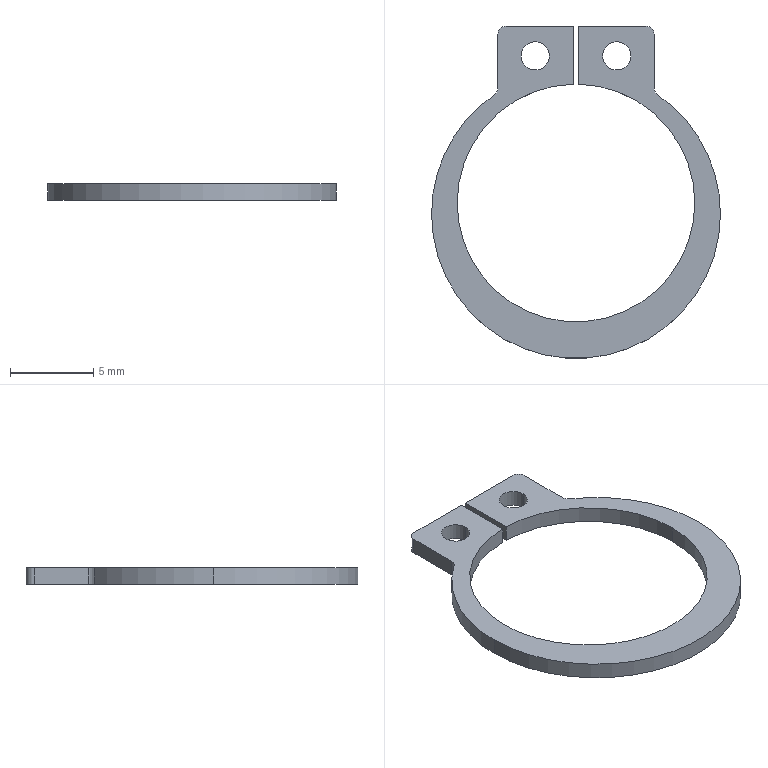Part | SolidWorks | features BaseBody 1 | 1 solid | 22 faces | box 17.38 x 20 x 1 mm | volume 99.766 mm3 | cylinder 14 | plane 8 | commonest cylinder face diameters 1 x4 1.7 x4 14.3 x3 17.38 x3
STEP:
#1=CARTESIAN_POINT('',(-130.796,1840.394,-232.));
#2=VERTEX_POINT('',#1);
#3=CARTESIAN_POINT('',(-129.096,1840.394,-232.));
#4=VERTEX_POINT('',#3);
#5=CARTESIAN_POINT('',(-129.946,1840.394,-232.));
#6=DIRECTION('',(0.,0.,1.));
#7=DIRECTION('',(1.,0.,0.));
#8=AXIS2_PLACEMENT_3D('',#5,#6,#7);
#9=CIRCLE('',#8,0.85);
#10=EDGE_CURVE('',#2,#4,#9,.T.);
#11=ORIENTED_EDGE('',*,*,#10,.F.);
#12=CARTESIAN_POINT('',(-130.796,1840.394,-231.));
#13=VERTEX_POINT('',#12);
#14=CARTESIAN_POINT('',(-130.796,1840.394,-232.));
#15=DIRECTION('',(0.,0.,1.));
#16=VECTOR('',#15,1000.);
#17=LINE('',#14,#16);
#18=EDGE_CURVE('',#2,#13,#17,.T.);
#19=ORIENTED_EDGE('',*,*,#18,.T.);
#20=CARTESIAN_POINT('',(-129.096,1840.394,-231.));
#21=VERTEX_POINT('',#20);
#22=CARTESIAN_POINT('',(-129.946,1840.394,-231.));
#23=DIRECTION('',(0.,0.,1.));
#24=DIRECTION('',(1.,0.,0.));
#25=AXIS2_PLACEMENT_3D('',#22,#23,#24);
#26=CIRCLE('',#25,0.85);
#27=EDGE_CURVE('',#13,#21,#26,.T.);
#28=ORIENTED_EDGE('',*,*,#27,.T.);
#29=CARTESIAN_POINT('',(-129.096,1840.394,-232.));
#30=DIRECTION('',(0.,0.,1.));
#31=VECTOR('',#30,1000.);
#32=LINE('',#29,#31);
#33=EDGE_CURVE('',#4,#21,#32,.T.);
#34=ORIENTED_EDGE('',*,*,#33,.F.);
#35=EDGE_LOOP('',(#11,#19,#28,#34));
#36=FACE_OUTER_BOUND('',#35,.T.);
#37=CARTESIAN_POINT('',(-129.946,1840.394,-232.));
#38=DIRECTION('',(0.,0.,1.));
#39=DIRECTION('',(1.,0.,0.));
#40=AXIS2_PLACEMENT_3D('',#37,#38,#39);
#41=CYLINDRICAL_SURFACE('',#40,0.85);
#42=ADVANCED_FACE('',(#36),#41,.F.);
#43=CARTESIAN_POINT('',(-125.896,1840.394,-232.));
#44=VERTEX_POINT('',#43);
#45=CARTESIAN_POINT('',(-124.196,1840.394,-232.));
#46=VERTEX_POINT('',#45);
#47=CARTESIAN_POINT('',(-125.046,1840.394,-232.));
#48=DIRECTION('',(0.,0.,1.));
#49=DIRECTION('',(1.,0.,0.));
#50=AXIS2_PLACEMENT_3D('',#47,#48,#49);
#51=CIRCLE('',#50,0.85);
#52=EDGE_CURVE('',#44,#46,#51,.T.);
#53=ORIENTED_EDGE('',*,*,#52,.F.);
#54=CARTESIAN_POINT('',(-125.896,1840.394,-231.));
#55=VERTEX_POINT('',#54);
#56=CARTESIAN_POINT('',(-125.896,1840.394,-232.));
#57=DIRECTION('',(0.,0.,1.));
#58=VECTOR('',#57,1000.);
#59=LINE('',#56,#58);
#60=EDGE_CURVE('',#44,#55,#59,.T.);
#61=ORIENTED_EDGE('',*,*,#60,.T.);
#62=CARTESIAN_POINT('',(-124.196,1840.394,-231.));
#63=VERTEX_POINT('',#62);
#64=CARTESIAN_POINT('',(-125.046,1840.394,-231.));
#65=DIRECTION('',(0.,0.,1.));
#66=DIRECTION('',(1.,0.,0.));
#67=AXIS2_PLACEMENT_3D('',#64,#65,#66);
#68=CIRCLE('',#67,0.85);
#69=EDGE_CURVE('',#55,#63,#68,.T.);
#70=ORIENTED_EDGE('',*,*,#69,.T.);
#71=CARTESIAN_POINT('',(-124.196,1840.394,-232.));
#72=DIRECTION('',(0.,0.,1.));
#73=VECTOR('',#72,1000.);
#74=LINE('',#71,#73);
#75=EDGE_CURVE('',#46,#63,#74,.T.);
#76=ORIENTED_EDGE('',*,*,#75,.F.);
#77=EDGE_LOOP('',(#53,#61,#70,#76));
#78=FACE_OUTER_BOUND('',#77,.T.);
#79=CARTESIAN_POINT('',(-125.046,1840.394,-232.));
#80=DIRECTION('',(0.,0.,1.));
#81=DIRECTION('',(1.,0.,0.));
#82=AXIS2_PLACEMENT_3D('',#79,#80,#81);
#83=CYLINDRICAL_SURFACE('',#82,0.85);
#84=ADVANCED_FACE('',(#78),#83,.F.);
#85=CARTESIAN_POINT('',(-132.413,1838.049,-232.));
#86=VERTEX_POINT('',#85);
#87=CARTESIAN_POINT('',(-136.186,1830.884,-232.));
#88=VERTEX_POINT('',#87);
#89=CARTESIAN_POINT('',(-127.496,1830.884,-232.));
#90=DIRECTION('',(0.,0.,1.));
#91=DIRECTION('',(1.,0.,0.));
#92=AXIS2_PLACEMENT_3D('',#89,#90,#91);
#93=CIRCLE('',#92,8.69);
#94=EDGE_CURVE('',#86,#88,#93,.T.);
#95=ORIENTED_EDGE('',*,*,#94,.T.);
#96=CARTESIAN_POINT('',(-136.186,1830.884,-231.));
#97=VERTEX_POINT('',#96);
#98=CARTESIAN_POINT('',(-136.186,1830.884,-232.));
#99=DIRECTION('',(0.,0.,1.));
#100=VECTOR('',#99,1000.);
#101=LINE('',#98,#100);
#102=EDGE_CURVE('',#88,#97,#101,.T.);
#103=ORIENTED_EDGE('',*,*,#102,.T.);
#104=CARTESIAN_POINT('',(-132.413,1838.049,-231.));
#105=VERTEX_POINT('',#104);
#106=CARTESIAN_POINT('',(-127.496,1830.884,-231.));
#107=DIRECTION('',(0.,0.,-1.));
#108=DIRECTION('',(1.,0.,0.));
#109=AXIS2_PLACEMENT_3D('',#106,#107,#108);
#110=CIRCLE('',#109,8.69);
#111=EDGE_CURVE('',#97,#105,#110,.T.);
#112=ORIENTED_EDGE('',*,*,#111,.T.);
#113=CARTESIAN_POINT('',(-132.413,1838.049,-232.));
#114=DIRECTION('',(0.,0.,-1.));
#115=VECTOR('',#114,1000.);
#116=LINE('',#113,#115);
#117=EDGE_CURVE('',#105,#86,#116,.T.);
#118=ORIENTED_EDGE('',*,*,#117,.T.);
#119=EDGE_LOOP('',(#95,#103,#112,#118));
#120=FACE_OUTER_BOUND('',#119,.T.);
#121=CARTESIAN_POINT('',(-127.496,1830.884,-232.));
#122=DIRECTION('',(0.,0.,1.));
#123=DIRECTION('',(1.,0.,0.));
#124=AXIS2_PLACEMENT_3D('',#121,#122,#123);
#125=CYLINDRICAL_SURFACE('',#124,8.69);
#126=ADVANCED_FACE('',(#120),#125,.T.);
#127=ORIENTED_EDGE('',*,*,#102,.F.);
#128=CARTESIAN_POINT('',(-118.806,1830.884,-232.));
#129=VERTEX_POINT('',#128);
#130=CARTESIAN_POINT('',(-127.496,1830.884,-232.));
#131=DIRECTION('',(0.,0.,1.));
#132=DIRECTION('',(1.,0.,0.));
#133=AXIS2_PLACEMENT_3D('',#130,#131,#132);
#134=CIRCLE('',#133,8.69);
#135=EDGE_CURVE('',#88,#129,#134,.T.);
#136=ORIENTED_EDGE('',*,*,#135,.T.);
#137=CARTESIAN_POINT('',(-118.806,1830.884,-231.));
#138=VERTEX_POINT('',#137);
#139=CARTESIAN_POINT('',(-118.806,1830.884,-232.));
#140=DIRECTION('',(0.,0.,1.));
#141=VECTOR('',#140,1000.);
#142=LINE('',#139,#141);
#143=EDGE_CURVE('',#129,#138,#142,.T.);
#144=ORIENTED_EDGE('',*,*,#143,.T.);
#145=CARTESIAN_POINT('',(-127.496,1830.884,-231.));
#146=DIRECTION('',(0.,0.,-1.));
#147=DIRECTION('',(1.,0.,0.));
#148=AXIS2_PLACEMENT_3D('',#145,#146,#147);
#149=CIRCLE('',#148,8.69);
#150=EDGE_CURVE('',#138,#97,#149,.T.);
#151=ORIENTED_EDGE('',*,*,#150,.T.);
#152=EDGE_LOOP('',(#127,#136,#144,#151));
#153=FACE_OUTER_BOUND('',#152,.T.);
#154=CARTESIAN_POINT('',(-127.496,1830.884,-232.));
#155=DIRECTION('',(0.,0.,1.));
#156=DIRECTION('',(1.,0.,0.));
#157=AXIS2_PLACEMENT_3D('',#154,#155,#156);
#158=CYLINDRICAL_SURFACE('',#157,8.69);
#159=ADVANCED_FACE('',(#153),#158,.T.);
#160=CARTESIAN_POINT('',(-134.646,1831.544,-232.));
#161=VERTEX_POINT('',#160);
#162=CARTESIAN_POINT('',(-120.346,1831.544,-232.));
#163=VERTEX_POINT('',#162);
#164=CARTESIAN_POINT('',(-127.496,1831.544,-232.));
#165=DIRECTION('',(0.,0.,1.));
#166=DIRECTION('',(1.,0.,0.));
#167=AXIS2_PLACEMENT_3D('',#164,#165,#166);
#168=CIRCLE('',#167,7.15);
#169=EDGE_CURVE('',#161,#163,#168,.T.);
#170=ORIENTED_EDGE('',*,*,#169,.F.);
#171=CARTESIAN_POINT('',(-134.646,1831.544,-231.));
#172=VERTEX_POINT('',#171);
#173=CARTESIAN_POINT('',(-134.646,1831.544,-232.));
#174=DIRECTION('',(0.,0.,1.));
#175=VECTOR('',#174,1000.);
#176=LINE('',#173,#175);
#177=EDGE_CURVE('',#161,#172,#176,.T.);
#178=ORIENTED_EDGE('',*,*,#177,.T.);
#179=CARTESIAN_POINT('',(-120.346,1831.544,-231.));
#180=VERTEX_POINT('',#179);
#181=CARTESIAN_POINT('',(-127.496,1831.544,-231.));
#182=DIRECTION('',(0.,0.,1.));
#183=DIRECTION('',(1.,0.,0.));
#184=AXIS2_PLACEMENT_3D('',#181,#182,#183);
#185=CIRCLE('',#184,7.15);
#186=EDGE_CURVE('',#172,#180,#185,.T.);
#187=ORIENTED_EDGE('',*,*,#186,.T.);
#188=CARTESIAN_POINT('',(-120.346,1831.544,-232.));
#189=DIRECTION('',(0.,0.,1.));
#190=VECTOR('',#189,1000.);
#191=LINE('',#188,#190);
#192=EDGE_CURVE('',#163,#180,#191,.T.);
#193=ORIENTED_EDGE('',*,*,#192,.F.);
#194=EDGE_LOOP('',(#170,#178,#187,#193));
#195=FACE_OUTER_BOUND('',#194,.T.);
#196=CARTESIAN_POINT('',(-127.496,1831.544,-232.));
#197=DIRECTION('',(0.,0.,1.));
#198=DIRECTION('',(1.,0.,0.));
#199=AXIS2_PLACEMENT_3D('',#196,#197,#198);
#200=CYLINDRICAL_SURFACE('',#199,7.15);
#201=ADVANCED_FACE('',(#195),#200,.F.);
#202=CARTESIAN_POINT('',(-127.346,1838.692,-232.));
#203=VERTEX_POINT('',#202);
#204=CARTESIAN_POINT('',(-127.496,1831.544,-232.));
#205=DIRECTION('',(0.,0.,1.));
#206=DIRECTION('',(1.,0.,0.));
#207=AXIS2_PLACEMENT_3D('',#204,#205,#206);
#208=CIRCLE('',#207,7.15);
#209=EDGE_CURVE('',#163,#203,#208,.T.);
#210=ORIENTED_EDGE('',*,*,#209,.F.);
#211=ORIENTED_EDGE('',*,*,#192,.T.);
#212=CARTESIAN_POINT('',(-127.346,1838.692,-231.));
#213=VERTEX_POINT('',#212);
#214=CARTESIAN_POINT('',(-127.496,1831.544,-231.));
#215=DIRECTION('',(0.,0.,1.));
#216=DIRECTION('',(1.,0.,0.));
#217=AXIS2_PLACEMENT_3D('',#214,#215,#216);
#218=CIRCLE('',#217,7.15);
#219=EDGE_CURVE('',#180,#213,#218,.T.);
#220=ORIENTED_EDGE('',*,*,#219,.T.);
#221=CARTESIAN_POINT('',(-127.346,1838.692,-232.));
#222=DIRECTION('',(0.,0.,1.));
#223=VECTOR('',#222,1000.);
#224=LINE('',#221,#223);
#225=EDGE_CURVE('',#203,#213,#224,.T.);
#226=ORIENTED_EDGE('',*,*,#225,.F.);
#227=EDGE_LOOP('',(#210,#211,#220,#226));
#228=FACE_OUTER_BOUND('',#227,.T.);
#229=CARTESIAN_POINT('',(-127.496,1831.544,-232.));
#230=DIRECTION('',(0.,0.,1.));
#231=DIRECTION('',(1.,0.,0.));
#232=AXIS2_PLACEMENT_3D('',#229,#230,#231);
#233=CYLINDRICAL_SURFACE('',#232,7.15);
#234=ADVANCED_FACE('',(#228),#233,.F.);
#235=CARTESIAN_POINT('',(-129.946,1840.394,-231.));
#236=DIRECTION('',(0.,0.,1.));
#237=DIRECTION('',(1.,0.,0.));
#238=AXIS2_PLACEMENT_3D('',#235,#236,#237);
#239=CIRCLE('',#238,0.85);
#240=EDGE_CURVE('',#21,#13,#239,.T.);
#241=ORIENTED_EDGE('',*,*,#240,.F.);
#242=ORIENTED_EDGE('',*,*,#27,.F.);
#243=EDGE_LOOP('',(#241,#242));
#244=FACE_BOUND('',#243,.T.);
#245=CARTESIAN_POINT('',(-125.046,1840.394,-231.));
#246=DIRECTION('',(0.,0.,1.));
#247=DIRECTION('',(1.,0.,0.));
#248=AXIS2_PLACEMENT_3D('',#245,#246,#247);
#249=CIRCLE('',#248,0.85);
#250=EDGE_CURVE('',#63,#55,#249,.T.);
#251=ORIENTED_EDGE('',*,*,#250,.F.);
#252=ORIENTED_EDGE('',*,*,#69,.F.);
#253=EDGE_LOOP('',(#251,#252));
#254=FACE_BOUND('',#253,.T.);
#255=CARTESIAN_POINT('',(-122.796,1838.461,-231.));
#256=VERTEX_POINT('',#255);
#257=CARTESIAN_POINT('',(-122.579,1838.049,-231.));
#258=VERTEX_POINT('',#257);
#259=CARTESIAN_POINT('',(-122.296,1838.461,-231.));
#260=DIRECTION('',(0.,0.,1.));
#261=DIRECTION('',(1.,0.,0.));
#262=AXIS2_PLACEMENT_3D('',#259,#260,#261);
#263=CIRCLE('',#262,0.5);
#264=EDGE_CURVE('',#256,#258,#263,.T.);
#265=ORIENTED_EDGE('',*,*,#264,.F.);
#266=CARTESIAN_POINT('',(-122.796,1841.694,-231.));
#267=VERTEX_POINT('',#266);
#268=CARTESIAN_POINT('',(-122.796,1838.461,-231.));
#269=DIRECTION('',(0.,-1.,0.));
#270=VECTOR('',#269,1000.);
#271=LINE('',#268,#270);
#272=EDGE_CURVE('',#267,#256,#271,.T.);
#273=ORIENTED_EDGE('',*,*,#272,.F.);
#274=CARTESIAN_POINT('',(-123.296,1842.194,-231.));
#275=VERTEX_POINT('',#274);
#276=CARTESIAN_POINT('',(-123.296,1841.694,-231.));
#277=DIRECTION('',(0.,0.,-1.));
#278=DIRECTION('',(1.,0.,0.));
#279=AXIS2_PLACEMENT_3D('',#276,#277,#278);
#280=CIRCLE('',#279,0.5);
#281=EDGE_CURVE('',#275,#267,#280,.T.);
#282=ORIENTED_EDGE('',*,*,#281,.F.);
#283=CARTESIAN_POINT('',(-127.346,1842.194,-231.));
#284=VERTEX_POINT('',#283);
#285=CARTESIAN_POINT('',(-132.696,1842.194,-231.));
#286=DIRECTION('',(1.,0.,0.));
#287=VECTOR('',#286,1000.);
#288=LINE('',#285,#287);
#289=EDGE_CURVE('',#284,#275,#288,.T.);
#290=ORIENTED_EDGE('',*,*,#289,.F.);
#291=CARTESIAN_POINT('',(-127.346,1838.461,-231.));
#292=DIRECTION('',(0.,1.,0.));
#293=VECTOR('',#292,1000.);
#294=LINE('',#291,#293);
#295=EDGE_CURVE('',#213,#284,#294,.T.);
#296=ORIENTED_EDGE('',*,*,#295,.F.);
#297=ORIENTED_EDGE('',*,*,#219,.F.);
#298=ORIENTED_EDGE('',*,*,#186,.F.);
#299=CARTESIAN_POINT('',(-127.646,1838.692,-231.));
#300=VERTEX_POINT('',#299);
#301=CARTESIAN_POINT('',(-127.496,1831.544,-231.));
#302=DIRECTION('',(0.,0.,1.));
#303=DIRECTION('',(1.,0.,0.));
#304=AXIS2_PLACEMENT_3D('',#301,#302,#303);
#305=CIRCLE('',#304,7.15);
#306=EDGE_CURVE('',#300,#172,#305,.T.);
#307=ORIENTED_EDGE('',*,*,#306,.F.);
#308=CARTESIAN_POINT('',(-127.646,1842.194,-231.));
#309=VERTEX_POINT('',#308);
#310=CARTESIAN_POINT('',(-127.646,1838.461,-231.));
#311=DIRECTION('',(0.,-1.,0.));
#312=VECTOR('',#311,1000.);
#313=LINE('',#310,#312);
#314=EDGE_CURVE('',#309,#300,#313,.T.);
#315=ORIENTED_EDGE('',*,*,#314,.F.);
#316=CARTESIAN_POINT('',(-131.696,1842.194,-231.));
#317=VERTEX_POINT('',#316);
#318=CARTESIAN_POINT('',(-132.696,1842.194,-231.));
#319=DIRECTION('',(1.,0.,0.));
#320=VECTOR('',#319,1000.);
#321=LINE('',#318,#320);
#322=EDGE_CURVE('',#317,#309,#321,.T.);
#323=ORIENTED_EDGE('',*,*,#322,.F.);
#324=CARTESIAN_POINT('',(-132.196,1841.694,-231.));
#325=VERTEX_POINT('',#324);
#326=CARTESIAN_POINT('',(-131.696,1841.694,-231.));
#327=DIRECTION('',(0.,0.,-1.));
#328=DIRECTION('',(1.,0.,0.));
#329=AXIS2_PLACEMENT_3D('',#326,#327,#328);
#330=CIRCLE('',#329,0.5);
#331=EDGE_CURVE('',#325,#317,#330,.T.);
#332=ORIENTED_EDGE('',*,*,#331,.F.);
#333=CARTESIAN_POINT('',(-132.196,1838.461,-231.));
#334=VERTEX_POINT('',#333);
#335=CARTESIAN_POINT('',(-132.196,1838.461,-231.));
#336=DIRECTION('',(0.,1.,0.));
#337=VECTOR('',#336,1000.);
#338=LINE('',#335,#337);
#339=EDGE_CURVE('',#334,#325,#338,.T.);
#340=ORIENTED_EDGE('',*,*,#339,.F.);
#341=CARTESIAN_POINT('',(-132.696,1838.461,-231.));
#342=DIRECTION('',(0.,0.,1.));
#343=DIRECTION('',(1.,0.,0.));
#344=AXIS2_PLACEMENT_3D('',#341,#342,#343);
#345=CIRCLE('',#344,0.5);
#346=EDGE_CURVE('',#105,#334,#345,.T.);
#347=ORIENTED_EDGE('',*,*,#346,.F.);
#348=ORIENTED_EDGE('',*,*,#111,.F.);
#349=ORIENTED_EDGE('',*,*,#150,.F.);
#350=CARTESIAN_POINT('',(-127.496,1830.884,-231.));
#351=DIRECTION('',(0.,0.,-1.));
#352=DIRECTION('',(1.,0.,0.));
#353=AXIS2_PLACEMENT_3D('',#350,#351,#352);
#354=CIRCLE('',#353,8.69);
#355=EDGE_CURVE('',#258,#138,#354,.T.);
#356=ORIENTED_EDGE('',*,*,#355,.F.);
#357=EDGE_LOOP('',(#265,#273,#282,#290,#296,#297,#298,#307,#315,#323,#332,#340,#347,#348,#349,#356));
#358=FACE_OUTER_BOUND('',#357,.T.);
#359=CARTESIAN_POINT('',(-132.696,1838.461,-231.));
#360=DIRECTION('',(0.,0.,-1.));
#361=DIRECTION('',(-1.,0.,0.));
#362=AXIS2_PLACEMENT_3D('',#359,#360,#361);
#363=PLANE('',#362);
#364=ADVANCED_FACE('',(#244,#254,#358),#363,.F.);
#365=ORIENTED_EDGE('',*,*,#18,.F.);
#366=CARTESIAN_POINT('',(-129.946,1840.394,-232.));
#367=DIRECTION('',(0.,0.,1.));
#368=DIRECTION('',(1.,0.,0.));
#369=AXIS2_PLACEMENT_3D('',#366,#367,#368);
#370=CIRCLE('',#369,0.85);
#371=EDGE_CURVE('',#4,#2,#370,.T.);
#372=ORIENTED_EDGE('',*,*,#371,.F.);
#373=ORIENTED_EDGE('',*,*,#33,.T.);
#374=ORIENTED_EDGE('',*,*,#240,.T.);
#375=EDGE_LOOP('',(#365,#372,#373,#374));
#376=FACE_OUTER_BOUND('',#375,.T.);
#377=CARTESIAN_POINT('',(-129.946,1840.394,-232.));
#378=DIRECTION('',(0.,0.,1.));
#379=DIRECTION('',(1.,0.,0.));
#380=AXIS2_PLACEMENT_3D('',#377,#378,#379);
#381=CYLINDRICAL_SURFACE('',#380,0.85);
#382=ADVANCED_FACE('',(#376),#381,.F.);
#383=ORIENTED_EDGE('',*,*,#60,.F.);
#384=CARTESIAN_POINT('',(-125.046,1840.394,-232.));
#385=DIRECTION('',(0.,0.,1.));
#386=DIRECTION('',(1.,0.,0.));
#387=AXIS2_PLACEMENT_3D('',#384,#385,#386);
#388=CIRCLE('',#387,0.85);
#389=EDGE_CURVE('',#46,#44,#388,.T.);
#390=ORIENTED_EDGE('',*,*,#389,.F.);
#391=ORIENTED_EDGE('',*,*,#75,.T.);
#392=ORIENTED_EDGE('',*,*,#250,.T.);
#393=EDGE_LOOP('',(#383,#390,#391,#392));
#394=FACE_OUTER_BOUND('',#393,.T.);
#395=CARTESIAN_POINT('',(-125.046,1840.394,-232.));
#396=DIRECTION('',(0.,0.,1.));
#397=DIRECTION('',(1.,0.,0.));
#398=AXIS2_PLACEMENT_3D('',#395,#396,#397);
#399=CYLINDRICAL_SURFACE('',#398,0.85);
#400=ADVANCED_FACE('',(#394),#399,.F.);
#401=ORIENTED_EDGE('',*,*,#143,.F.);
#402=CARTESIAN_POINT('',(-122.579,1838.049,-232.));
#403=VERTEX_POINT('',#402);
#404=CARTESIAN_POINT('',(-127.496,1830.884,-232.));
#405=DIRECTION('',(0.,0.,1.));
#406=DIRECTION('',(1.,0.,0.));
#407=AXIS2_PLACEMENT_3D('',#404,#405,#406);
#408=CIRCLE('',#407,8.69);
#409=EDGE_CURVE('',#129,#403,#408,.T.);
#410=ORIENTED_EDGE('',*,*,#409,.T.);
#411=CARTESIAN_POINT('',(-122.579,1838.049,-232.));
#412=DIRECTION('',(0.,0.,1.));
#413=VECTOR('',#412,1000.);
#414=LINE('',#411,#413);
#415=EDGE_CURVE('',#403,#258,#414,.T.);
#416=ORIENTED_EDGE('',*,*,#415,.T.);
#417=ORIENTED_EDGE('',*,*,#355,.T.);
#418=EDGE_LOOP('',(#401,#410,#416,#417));
#419=FACE_OUTER_BOUND('',#418,.T.);
#420=CARTESIAN_POINT('',(-127.496,1830.884,-232.));
#421=DIRECTION('',(0.,0.,1.));
#422=DIRECTION('',(1.,0.,0.));
#423=AXIS2_PLACEMENT_3D('',#420,#421,#422);
#424=CYLINDRICAL_SURFACE('',#423,8.69);
#425=ADVANCED_FACE('',(#419),#424,.T.);
#426=CARTESIAN_POINT('',(-122.796,1838.461,-232.));
#427=VERTEX_POINT('',#426);
#428=CARTESIAN_POINT('',(-122.296,1838.461,-232.));
#429=DIRECTION('',(0.,0.,1.));
#430=DIRECTION('',(1.,0.,0.));
#431=AXIS2_PLACEMENT_3D('',#428,#429,#430);
#432=CIRCLE('',#431,0.5);
#433=EDGE_CURVE('',#427,#403,#432,.T.);
#434=ORIENTED_EDGE('',*,*,#433,.F.);
#435=CARTESIAN_POINT('',(-122.796,1838.461,-232.));
#436=DIRECTION('',(0.,0.,-1.));
#437=VECTOR('',#436,1000.);
#438=LINE('',#435,#437);
#439=EDGE_CURVE('',#256,#427,#438,.T.);
#440=ORIENTED_EDGE('',*,*,#439,.F.);
#441=ORIENTED_EDGE('',*,*,#264,.T.);
#442=ORIENTED_EDGE('',*,*,#415,.F.);
#443=EDGE_LOOP('',(#434,#440,#441,#442));
#444=FACE_OUTER_BOUND('',#443,.T.);
#445=CARTESIAN_POINT('',(-122.296,1838.461,-232.));
#446=DIRECTION('',(0.,0.,1.));
#447=DIRECTION('',(1.,0.,0.));
#448=AXIS2_PLACEMENT_3D('',#445,#446,#447);
#449=CYLINDRICAL_SURFACE('',#448,0.5);
#450=ADVANCED_FACE('',(#444),#449,.F.);
#451=CARTESIAN_POINT('',(-122.796,1841.694,-232.));
#452=VERTEX_POINT('',#451);
#453=CARTESIAN_POINT('',(-122.796,1841.694,-232.));
#454=DIRECTION('',(0.,0.,1.));
#455=VECTOR('',#454,1000.);
#456=LINE('',#453,#455);
#457=EDGE_CURVE('',#452,#267,#456,.T.);
#458=ORIENTED_EDGE('',*,*,#457,.T.);
#459=ORIENTED_EDGE('',*,*,#272,.T.);
#460=ORIENTED_EDGE('',*,*,#439,.T.);
#461=CARTESIAN_POINT('',(-122.796,1838.461,-232.));
#462=DIRECTION('',(0.,1.,0.));
#463=VECTOR('',#462,1000.);
#464=LINE('',#461,#463);
#465=EDGE_CURVE('',#427,#452,#464,.T.);
#466=ORIENTED_EDGE('',*,*,#465,.T.);
#467=EDGE_LOOP('',(#458,#459,#460,#466));
#468=FACE_OUTER_BOUND('',#467,.T.);
#469=CARTESIAN_POINT('',(-122.796,1838.461,-232.));
#470=DIRECTION('',(1.,0.,0.));
#471=DIRECTION('',(0.,0.,-1.));
#472=AXIS2_PLACEMENT_3D('',#469,#470,#471);
#473=PLANE('',#472);
#474=ADVANCED_FACE('',(#468),#473,.T.);
#475=CARTESIAN_POINT('',(-123.296,1842.194,-232.));
#476=VERTEX_POINT('',#475);
#477=CARTESIAN_POINT('',(-123.296,1842.194,-232.));
#478=DIRECTION('',(0.,0.,1.));
#479=VECTOR('',#478,1000.);
#480=LINE('',#477,#479);
#481=EDGE_CURVE('',#476,#275,#480,.T.);
#482=ORIENTED_EDGE('',*,*,#481,.T.);
#483=ORIENTED_EDGE('',*,*,#281,.T.);
#484=ORIENTED_EDGE('',*,*,#457,.F.);
#485=CARTESIAN_POINT('',(-123.296,1841.694,-232.));
#486=DIRECTION('',(0.,0.,1.));
#487=DIRECTION('',(1.,0.,0.));
#488=AXIS2_PLACEMENT_3D('',#485,#486,#487);
#489=CIRCLE('',#488,0.5);
#490=EDGE_CURVE('',#452,#476,#489,.T.);
#491=ORIENTED_EDGE('',*,*,#490,.T.);
#492=EDGE_LOOP('',(#482,#483,#484,#491));
#493=FACE_OUTER_BOUND('',#492,.T.);
#494=CARTESIAN_POINT('',(-123.296,1841.694,-232.));
#495=DIRECTION('',(0.,0.,1.));
#496=DIRECTION('',(1.,0.,0.));
#497=AXIS2_PLACEMENT_3D('',#494,#495,#496);
#498=CYLINDRICAL_SURFACE('',#497,0.5);
#499=ADVANCED_FACE('',(#493),#498,.T.);
#500=CARTESIAN_POINT('',(-127.346,1842.194,-232.));
#501=VERTEX_POINT('',#500);
#502=CARTESIAN_POINT('',(-127.346,1842.194,-232.));
#503=DIRECTION('',(0.,0.,1.));
#504=VECTOR('',#503,1000.);
#505=LINE('',#502,#504);
#506=EDGE_CURVE('',#501,#284,#505,.T.);
#507=ORIENTED_EDGE('',*,*,#506,.T.);
#508=ORIENTED_EDGE('',*,*,#289,.T.);
#509=ORIENTED_EDGE('',*,*,#481,.F.);
#510=CARTESIAN_POINT('',(-123.296,1842.194,-232.));
#511=DIRECTION('',(-1.,0.,0.));
#512=VECTOR('',#511,1000.);
#513=LINE('',#510,#512);
#514=EDGE_CURVE('',#476,#501,#513,.T.);
#515=ORIENTED_EDGE('',*,*,#514,.T.);
#516=EDGE_LOOP('',(#507,#508,#509,#515));
#517=FACE_OUTER_BOUND('',#516,.T.);
#518=CARTESIAN_POINT('',(-123.296,1842.194,-232.));
#519=DIRECTION('',(0.,1.,0.));
#520=DIRECTION('',(0.,0.,1.));
#521=AXIS2_PLACEMENT_3D('',#518,#519,#520);
#522=PLANE('',#521);
#523=ADVANCED_FACE('',(#517),#522,.T.);
#524=ORIENTED_EDGE('',*,*,#225,.T.);
#525=ORIENTED_EDGE('',*,*,#295,.T.);
#526=ORIENTED_EDGE('',*,*,#506,.F.);
#527=CARTESIAN_POINT('',(-127.346,1842.194,-232.));
#528=DIRECTION('',(0.,-1.,0.));
#529=VECTOR('',#528,1000.);
#530=LINE('',#527,#529);
#531=EDGE_CURVE('',#501,#203,#530,.T.);
#532=ORIENTED_EDGE('',*,*,#531,.T.);
#533=EDGE_LOOP('',(#524,#525,#526,#532));
#534=FACE_OUTER_BOUND('',#533,.T.);
#535=CARTESIAN_POINT('',(-127.346,1842.194,-232.));
#536=DIRECTION('',(-1.,0.,0.));
#537=DIRECTION('',(0.,0.,1.));
#538=AXIS2_PLACEMENT_3D('',#535,#536,#537);
#539=PLANE('',#538);
#540=ADVANCED_FACE('',(#534),#539,.T.);
#541=ORIENTED_EDGE('',*,*,#177,.F.);
#542=CARTESIAN_POINT('',(-127.646,1838.692,-232.));
#543=VERTEX_POINT('',#542);
#544=CARTESIAN_POINT('',(-127.496,1831.544,-232.));
#545=DIRECTION('',(0.,0.,1.));
#546=DIRECTION('',(1.,0.,0.));
#547=AXIS2_PLACEMENT_3D('',#544,#545,#546);
#548=CIRCLE('',#547,7.15);
#549=EDGE_CURVE('',#543,#161,#548,.T.);
#550=ORIENTED_EDGE('',*,*,#549,.F.);
#551=CARTESIAN_POINT('',(-127.646,1838.692,-232.));
#552=DIRECTION('',(0.,0.,-1.));
#553=VECTOR('',#552,1000.);
#554=LINE('',#551,#553);
#555=EDGE_CURVE('',#300,#543,#554,.T.);
#556=ORIENTED_EDGE('',*,*,#555,.F.);
#557=ORIENTED_EDGE('',*,*,#306,.T.);
#558=EDGE_LOOP('',(#541,#550,#556,#557));
#559=FACE_OUTER_BOUND('',#558,.T.);
#560=CARTESIAN_POINT('',(-127.496,1831.544,-232.));
#561=DIRECTION('',(0.,0.,1.));
#562=DIRECTION('',(1.,0.,0.));
#563=AXIS2_PLACEMENT_3D('',#560,#561,#562);
#564=CYLINDRICAL_SURFACE('',#563,7.15);
#565=ADVANCED_FACE('',(#559),#564,.F.);
#566=CARTESIAN_POINT('',(-127.646,1842.194,-232.));
#567=VERTEX_POINT('',#566);
#568=CARTESIAN_POINT('',(-127.646,1842.194,-232.));
#569=DIRECTION('',(0.,0.,1.));
#570=VECTOR('',#569,1000.);
#571=LINE('',#568,#570);
#572=EDGE_CURVE('',#567,#309,#571,.T.);
#573=ORIENTED_EDGE('',*,*,#572,.T.);
#574=ORIENTED_EDGE('',*,*,#314,.T.);
#575=ORIENTED_EDGE('',*,*,#555,.T.);
#576=CARTESIAN_POINT('',(-127.646,1838.692,-232.));
#577=DIRECTION('',(0.,1.,0.));
#578=VECTOR('',#577,1000.);
#579=LINE('',#576,#578);
#580=EDGE_CURVE('',#543,#567,#579,.T.);
#581=ORIENTED_EDGE('',*,*,#580,.T.);
#582=EDGE_LOOP('',(#573,#574,#575,#581));
#583=FACE_OUTER_BOUND('',#582,.T.);
#584=CARTESIAN_POINT('',(-127.646,1838.692,-232.));
#585=DIRECTION('',(1.,0.,0.));
#586=DIRECTION('',(0.,0.,-1.));
#587=AXIS2_PLACEMENT_3D('',#584,#585,#586);
#588=PLANE('',#587);
#589=ADVANCED_FACE('',(#583),#588,.T.);
#590=CARTESIAN_POINT('',(-131.696,1842.194,-232.));
#591=VERTEX_POINT('',#590);
#592=CARTESIAN_POINT('',(-131.696,1842.194,-232.));
#593=DIRECTION('',(0.,0.,1.));
#594=VECTOR('',#593,1000.);
#595=LINE('',#592,#594);
#596=EDGE_CURVE('',#591,#317,#595,.T.);
#597=ORIENTED_EDGE('',*,*,#596,.T.);
#598=ORIENTED_EDGE('',*,*,#322,.T.);
#599=ORIENTED_EDGE('',*,*,#572,.F.);
#600=CARTESIAN_POINT('',(-127.646,1842.194,-232.));
#601=DIRECTION('',(-1.,0.,0.));
#602=VECTOR('',#601,1000.);
#603=LINE('',#600,#602);
#604=EDGE_CURVE('',#567,#591,#603,.T.);
#605=ORIENTED_EDGE('',*,*,#604,.T.);
#606=EDGE_LOOP('',(#597,#598,#599,#605));
#607=FACE_OUTER_BOUND('',#606,.T.);
#608=CARTESIAN_POINT('',(-127.646,1842.194,-232.));
#609=DIRECTION('',(0.,1.,0.));
#610=DIRECTION('',(0.,0.,1.));
#611=AXIS2_PLACEMENT_3D('',#608,#609,#610);
#612=PLANE('',#611);
#613=ADVANCED_FACE('',(#607),#612,.T.);
#614=CARTESIAN_POINT('',(-132.196,1841.694,-232.));
#615=VERTEX_POINT('',#614);
#616=CARTESIAN_POINT('',(-132.196,1841.694,-232.));
#617=DIRECTION('',(0.,0.,1.));
#618=VECTOR('',#617,1000.);
#619=LINE('',#616,#618);
#620=EDGE_CURVE('',#615,#325,#619,.T.);
#621=ORIENTED_EDGE('',*,*,#620,.T.);
#622=ORIENTED_EDGE('',*,*,#331,.T.);
#623=ORIENTED_EDGE('',*,*,#596,.F.);
#624=CARTESIAN_POINT('',(-131.696,1841.694,-232.));
#625=DIRECTION('',(0.,0.,1.));
#626=DIRECTION('',(1.,0.,0.));
#627=AXIS2_PLACEMENT_3D('',#624,#625,#626);
#628=CIRCLE('',#627,0.5);
#629=EDGE_CURVE('',#591,#615,#628,.T.);
#630=ORIENTED_EDGE('',*,*,#629,.T.);
#631=EDGE_LOOP('',(#621,#622,#623,#630));
#632=FACE_OUTER_BOUND('',#631,.T.);
#633=CARTESIAN_POINT('',(-131.696,1841.694,-232.));
#634=DIRECTION('',(0.,0.,1.));
#635=DIRECTION('',(1.,0.,0.));
#636=AXIS2_PLACEMENT_3D('',#633,#634,#635);
#637=CYLINDRICAL_SURFACE('',#636,0.5);
#638=ADVANCED_FACE('',(#632),#637,.T.);
#639=CARTESIAN_POINT('',(-132.196,1838.461,-232.));
#640=VERTEX_POINT('',#639);
#641=CARTESIAN_POINT('',(-132.196,1838.461,-232.));
#642=DIRECTION('',(0.,0.,1.));
#643=VECTOR('',#642,1000.);
#644=LINE('',#641,#643);
#645=EDGE_CURVE('',#640,#334,#644,.T.);
#646=ORIENTED_EDGE('',*,*,#645,.T.);
#647=ORIENTED_EDGE('',*,*,#339,.T.);
#648=ORIENTED_EDGE('',*,*,#620,.F.);
#649=CARTESIAN_POINT('',(-132.196,1841.694,-232.));
#650=DIRECTION('',(0.,-1.,0.));
#651=VECTOR('',#650,1000.);
#652=LINE('',#649,#651);
#653=EDGE_CURVE('',#615,#640,#652,.T.);
#654=ORIENTED_EDGE('',*,*,#653,.T.);
#655=EDGE_LOOP('',(#646,#647,#648,#654));
#656=FACE_OUTER_BOUND('',#655,.T.);
#657=CARTESIAN_POINT('',(-132.196,1841.694,-232.));
#658=DIRECTION('',(-1.,0.,0.));
#659=DIRECTION('',(0.,0.,1.));
#660=AXIS2_PLACEMENT_3D('',#657,#658,#659);
#661=PLANE('',#660);
#662=ADVANCED_FACE('',(#656),#661,.T.);
#663=CARTESIAN_POINT('',(-132.696,1838.461,-232.));
#664=DIRECTION('',(0.,0.,1.));
#665=DIRECTION('',(1.,0.,0.));
#666=AXIS2_PLACEMENT_3D('',#663,#664,#665);
#667=CIRCLE('',#666,0.5);
#668=EDGE_CURVE('',#86,#640,#667,.T.);
#669=ORIENTED_EDGE('',*,*,#668,.F.);
#670=ORIENTED_EDGE('',*,*,#117,.F.);
#671=ORIENTED_EDGE('',*,*,#346,.T.);
#672=ORIENTED_EDGE('',*,*,#645,.F.);
#673=EDGE_LOOP('',(#669,#670,#671,#672));
#674=FACE_OUTER_BOUND('',#673,.T.);
#675=CARTESIAN_POINT('',(-132.696,1838.461,-232.));
#676=DIRECTION('',(0.,0.,1.));
#677=DIRECTION('',(1.,0.,0.));
#678=AXIS2_PLACEMENT_3D('',#675,#676,#677);
#679=CYLINDRICAL_SURFACE('',#678,0.5);
#680=ADVANCED_FACE('',(#674),#679,.F.);
#681=ORIENTED_EDGE('',*,*,#371,.T.);
#682=ORIENTED_EDGE('',*,*,#10,.T.);
#683=EDGE_LOOP('',(#681,#682));
#684=FACE_BOUND('',#683,.T.);
#685=ORIENTED_EDGE('',*,*,#389,.T.);
#686=ORIENTED_EDGE('',*,*,#52,.T.);
#687=EDGE_LOOP('',(#685,#686));
#688=FACE_BOUND('',#687,.T.);
#689=ORIENTED_EDGE('',*,*,#94,.F.);
#690=ORIENTED_EDGE('',*,*,#668,.T.);
#691=ORIENTED_EDGE('',*,*,#653,.F.);
#692=ORIENTED_EDGE('',*,*,#629,.F.);
#693=ORIENTED_EDGE('',*,*,#604,.F.);
#694=ORIENTED_EDGE('',*,*,#580,.F.);
#695=ORIENTED_EDGE('',*,*,#549,.T.);
#696=ORIENTED_EDGE('',*,*,#169,.T.);
#697=ORIENTED_EDGE('',*,*,#209,.T.);
#698=ORIENTED_EDGE('',*,*,#531,.F.);
#699=ORIENTED_EDGE('',*,*,#514,.F.);
#700=ORIENTED_EDGE('',*,*,#490,.F.);
#701=ORIENTED_EDGE('',*,*,#465,.F.);
#702=ORIENTED_EDGE('',*,*,#433,.T.);
#703=ORIENTED_EDGE('',*,*,#409,.F.);
#704=ORIENTED_EDGE('',*,*,#135,.F.);
#705=EDGE_LOOP('',(#689,#690,#691,#692,#693,#694,#695,#696,#697,#698,#699,#700,#701,#702,#703,#704));
#706=FACE_OUTER_BOUND('',#705,.T.);
#707=CARTESIAN_POINT('',(-132.696,1838.461,-232.));
#708=DIRECTION('',(0.,0.,-1.));
#709=DIRECTION('',(-1.,0.,0.));
#710=AXIS2_PLACEMENT_3D('',#707,#708,#709);
#711=PLANE('',#710);
#712=ADVANCED_FACE('',(#684,#688,#706),#711,.T.);
#713=CLOSED_SHELL('',(#42,#84,#126,#159,#201,#234,#364,#382,#400,#425,#450,#474,#499,#523,#540,#565,#589,#613,#638,#662,#680,#712));
#714=MANIFOLD_SOLID_BREP('',#713);
#715=CARTESIAN_POINT('',(0.,0.,0.));
#716=DIRECTION('',(0.,0.,1.));
#717=DIRECTION('',(1.,0.,0.));
#718=AXIS2_PLACEMENT_3D('',#715,#716,#717);
#719=(LENGTH_UNIT()NAMED_UNIT(*)SI_UNIT(.MILLI.,.METRE.));
#720=UNCERTAINTY_MEASURE_WITH_UNIT(LENGTH_MEASURE(0.00001),#719,'','');
#721=(NAMED_UNIT(*)PLANE_ANGLE_UNIT()SI_UNIT($,.RADIAN.));
#722=(NAMED_UNIT(*)SI_UNIT($,.STERADIAN.)SOLID_ANGLE_UNIT());
#723=(GEOMETRIC_REPRESENTATION_CONTEXT(3)GLOBAL_UNCERTAINTY_ASSIGNED_CONTEXT((#720))GLOBAL_UNIT_ASSIGNED_CONTEXT((#719,#721,#722))REPRESENTATION_CONTEXT('',''));
#724=ADVANCED_BREP_SHAPE_REPRESENTATION('',(#714,#718),#723);